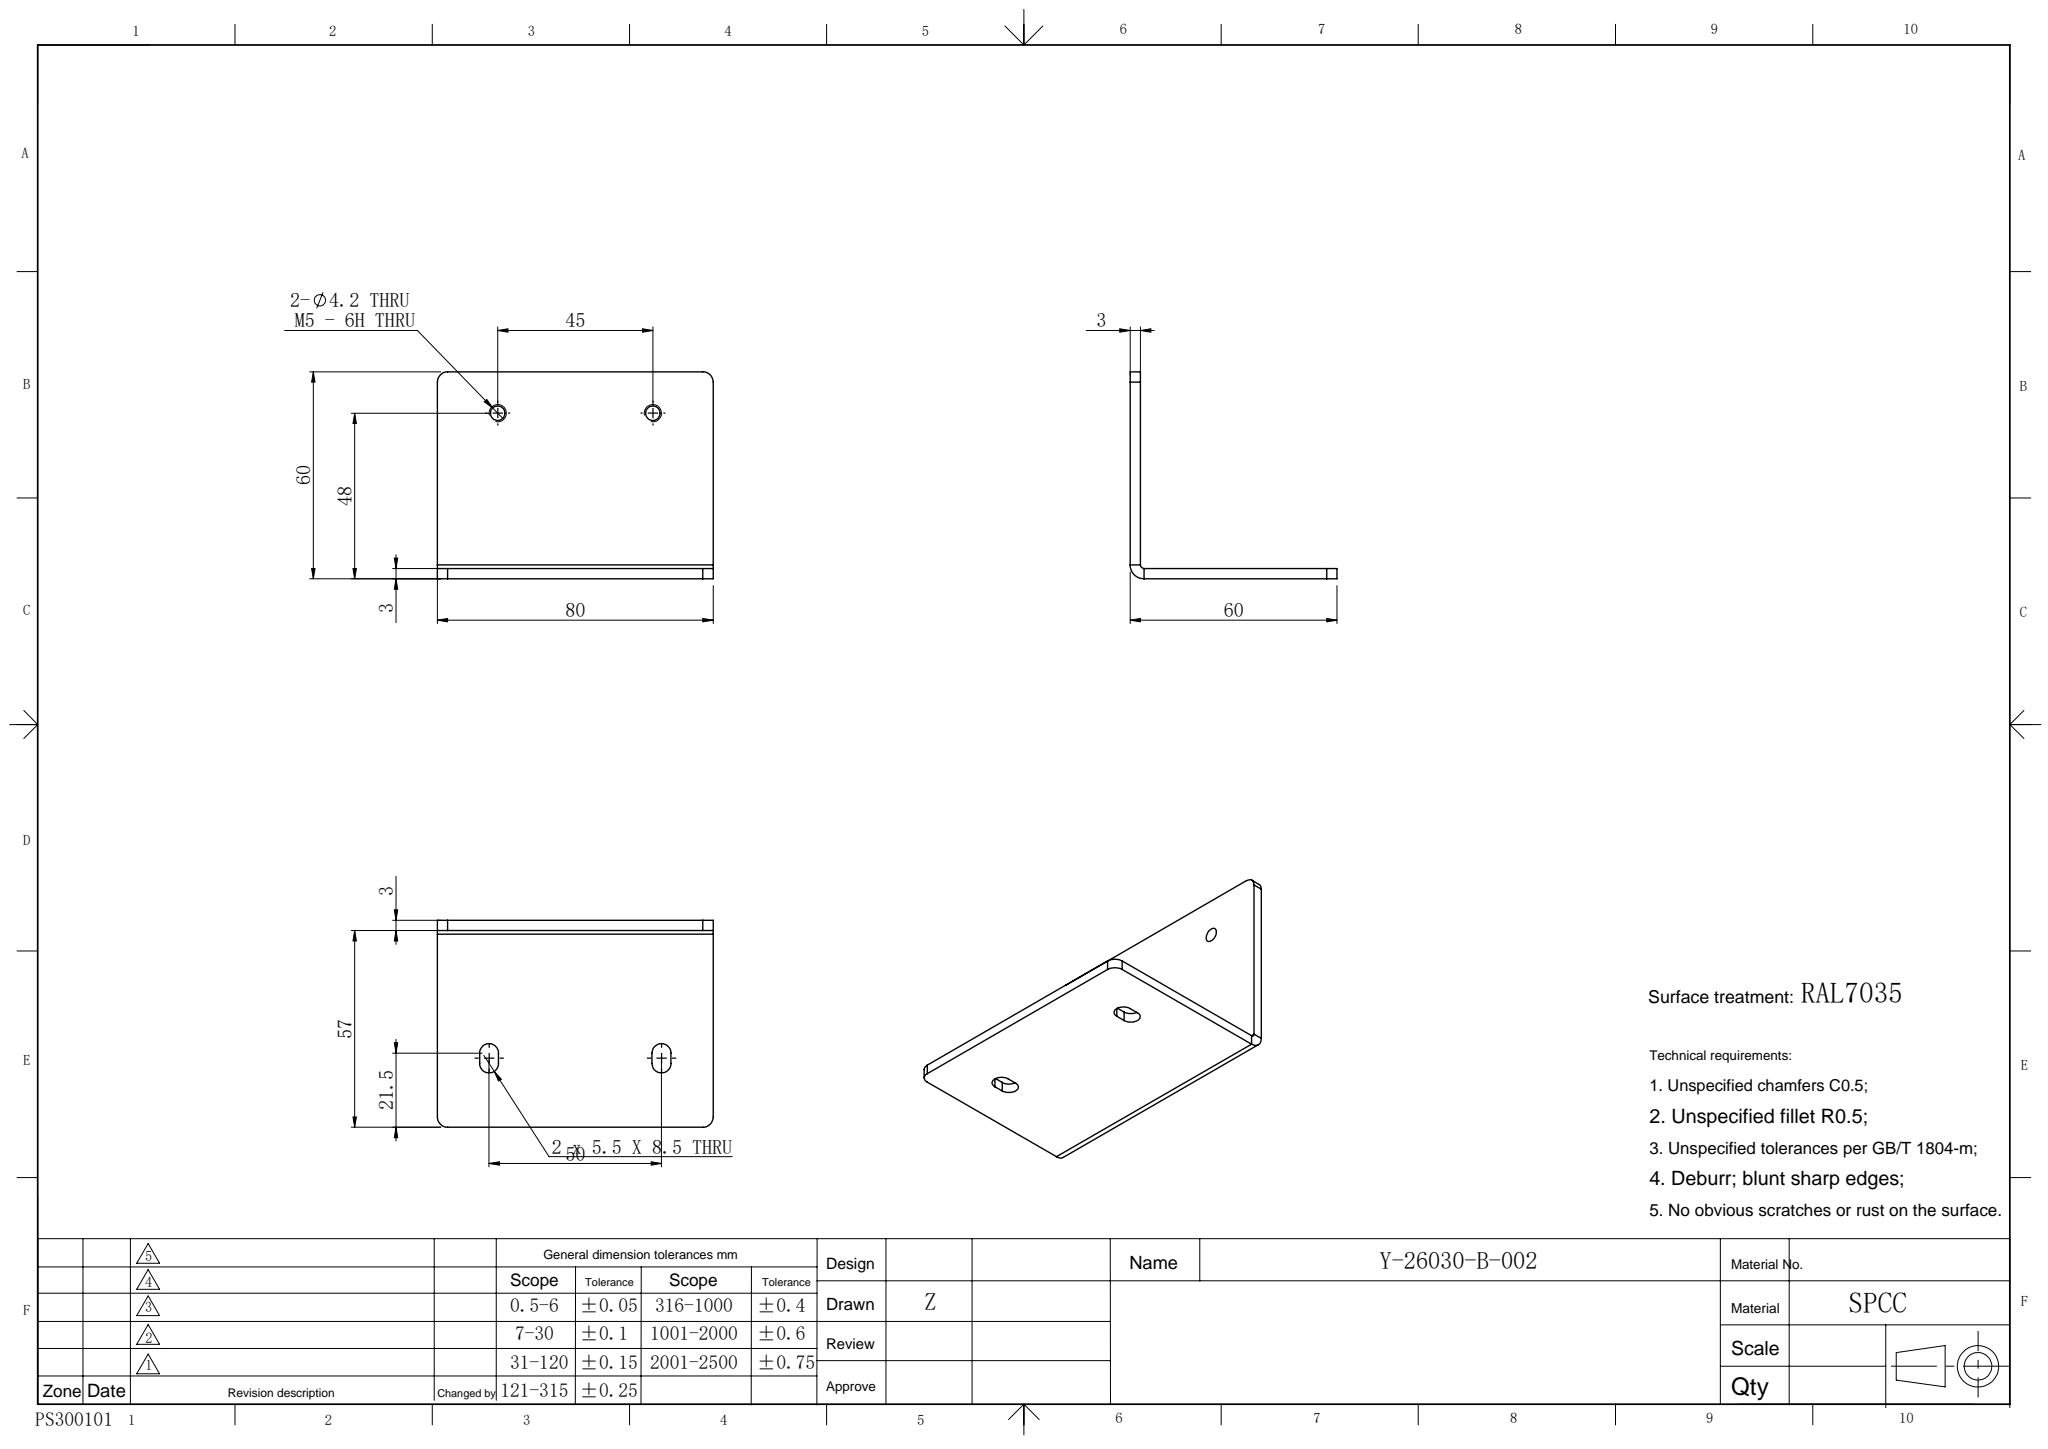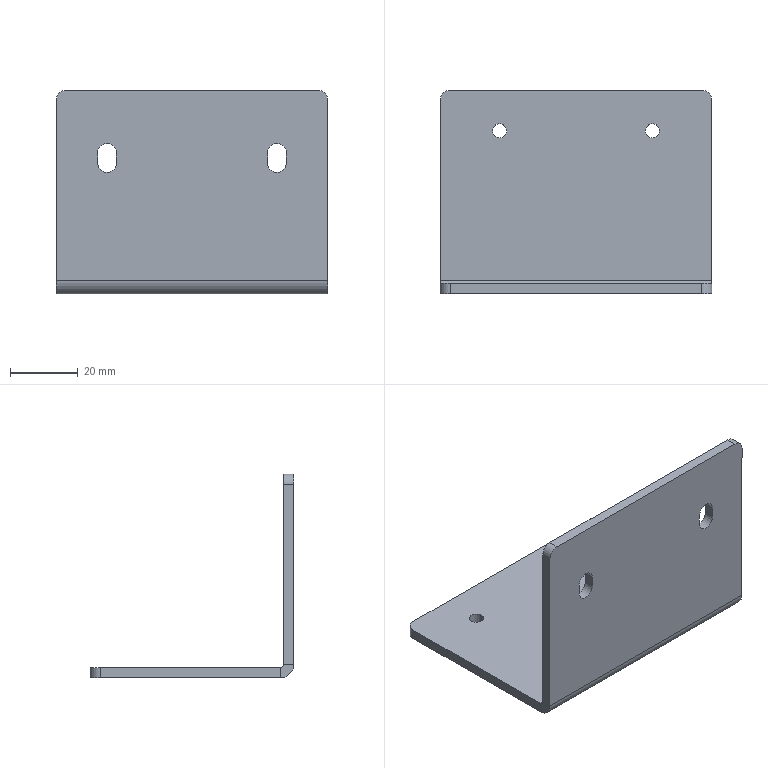Part | SolidWorks | features HoleWzd 2, EdgeFlange 1, Fillet 1, FlatPattern 1, SMBaseFlange 1, SheetMetal 1 | 1 solid | 32 faces | box 80 x 60 x 60 mm | volume 27475 mm3 | cylinder 16 | plane 16 | commonest cylinder face diameters 5.5 x6 4.2 x4 6 x4 2 x1 8 x1
STEP:
#1=CARTESIAN_POINT('',(-25.,-30.,41.25));
#2=VERTEX_POINT('',#1);
#3=CARTESIAN_POINT('',(-22.25,-30.,38.5));
#4=VERTEX_POINT('',#3);
#5=CARTESIAN_POINT('',(-25.,-30.,38.5));
#6=DIRECTION('',(0.,1.,0.));
#7=DIRECTION('',(0.,0.,1.));
#8=AXIS2_PLACEMENT_3D('',#5,#6,#7);
#9=CIRCLE('',#8,2.75);
#10=EDGE_CURVE('',#2,#4,#9,.T.);
#11=ORIENTED_EDGE('',*,*,#10,.F.);
#12=CARTESIAN_POINT('',(-25.,-27.,41.25));
#13=VERTEX_POINT('',#12);
#14=CARTESIAN_POINT('',(-25.,-27.,41.25));
#15=DIRECTION('',(0.,1.,0.));
#16=VECTOR('',#15,1000.);
#17=LINE('',#14,#16);
#18=EDGE_CURVE('',#2,#13,#17,.T.);
#19=ORIENTED_EDGE('',*,*,#18,.T.);
#20=CARTESIAN_POINT('',(-22.25,-27.,38.5));
#21=VERTEX_POINT('',#20);
#22=CARTESIAN_POINT('',(-25.,-27.,38.5));
#23=DIRECTION('',(0.,1.,0.));
#24=DIRECTION('',(0.,0.,1.));
#25=AXIS2_PLACEMENT_3D('',#22,#23,#24);
#26=CIRCLE('',#25,2.75);
#27=EDGE_CURVE('',#13,#21,#26,.T.);
#28=ORIENTED_EDGE('',*,*,#27,.T.);
#29=CARTESIAN_POINT('',(-22.25,-30.001,38.5));
#30=DIRECTION('',(0.,-1.,0.));
#31=VECTOR('',#30,1000.);
#32=LINE('',#29,#31);
#33=EDGE_CURVE('',#21,#4,#32,.T.);
#34=ORIENTED_EDGE('',*,*,#33,.T.);
#35=EDGE_LOOP('',(#11,#19,#28,#34));
#36=FACE_OUTER_BOUND('',#35,.T.);
#37=CARTESIAN_POINT('',(-25.,-27.,38.5));
#38=DIRECTION('',(0.,1.,0.));
#39=DIRECTION('',(0.,0.,1.));
#40=AXIS2_PLACEMENT_3D('',#37,#38,#39);
#41=CYLINDRICAL_SURFACE('',#40,2.75);
#42=ADVANCED_FACE('',(#36),#41,.F.);
#43=CARTESIAN_POINT('',(25.,-30.,41.25));
#44=VERTEX_POINT('',#43);
#45=CARTESIAN_POINT('',(27.75,-30.,38.5));
#46=VERTEX_POINT('',#45);
#47=CARTESIAN_POINT('',(25.,-30.,38.5));
#48=DIRECTION('',(0.,1.,0.));
#49=DIRECTION('',(0.,0.,1.));
#50=AXIS2_PLACEMENT_3D('',#47,#48,#49);
#51=CIRCLE('',#50,2.75);
#52=EDGE_CURVE('',#44,#46,#51,.T.);
#53=ORIENTED_EDGE('',*,*,#52,.F.);
#54=CARTESIAN_POINT('',(25.,-27.,41.25));
#55=VERTEX_POINT('',#54);
#56=CARTESIAN_POINT('',(25.,-27.,41.25));
#57=DIRECTION('',(0.,1.,0.));
#58=VECTOR('',#57,1000.);
#59=LINE('',#56,#58);
#60=EDGE_CURVE('',#44,#55,#59,.T.);
#61=ORIENTED_EDGE('',*,*,#60,.T.);
#62=CARTESIAN_POINT('',(27.75,-27.,38.5));
#63=VERTEX_POINT('',#62);
#64=CARTESIAN_POINT('',(25.,-27.,38.5));
#65=DIRECTION('',(0.,1.,0.));
#66=DIRECTION('',(0.,0.,1.));
#67=AXIS2_PLACEMENT_3D('',#64,#65,#66);
#68=CIRCLE('',#67,2.75);
#69=EDGE_CURVE('',#55,#63,#68,.T.);
#70=ORIENTED_EDGE('',*,*,#69,.T.);
#71=CARTESIAN_POINT('',(27.75,-30.001,38.5));
#72=DIRECTION('',(0.,-1.,0.));
#73=VECTOR('',#72,1000.);
#74=LINE('',#71,#73);
#75=EDGE_CURVE('',#63,#46,#74,.T.);
#76=ORIENTED_EDGE('',*,*,#75,.T.);
#77=EDGE_LOOP('',(#53,#61,#70,#76));
#78=FACE_OUTER_BOUND('',#77,.T.);
#79=CARTESIAN_POINT('',(25.,-27.,38.5));
#80=DIRECTION('',(0.,1.,0.));
#81=DIRECTION('',(0.,0.,1.));
#82=AXIS2_PLACEMENT_3D('',#79,#80,#81);
#83=CYLINDRICAL_SURFACE('',#82,2.75);
#84=ADVANCED_FACE('',(#78),#83,.F.);
#85=CARTESIAN_POINT('',(20.4,18.,0.));
#86=VERTEX_POINT('',#85);
#87=CARTESIAN_POINT('',(24.6,18.,0.));
#88=VERTEX_POINT('',#87);
#89=CARTESIAN_POINT('',(22.5,18.,0.));
#90=DIRECTION('',(0.,0.,1.));
#91=DIRECTION('',(1.,0.,0.));
#92=AXIS2_PLACEMENT_3D('',#89,#90,#91);
#93=CIRCLE('',#92,2.1);
#94=EDGE_CURVE('',#86,#88,#93,.T.);
#95=ORIENTED_EDGE('',*,*,#94,.T.);
#96=CARTESIAN_POINT('',(24.6,18.,-3.));
#97=VERTEX_POINT('',#96);
#98=CARTESIAN_POINT('',(24.6,18.,-3.));
#99=DIRECTION('',(0.,0.,-1.));
#100=VECTOR('',#99,1000.);
#101=LINE('',#98,#100);
#102=EDGE_CURVE('',#88,#97,#101,.T.);
#103=ORIENTED_EDGE('',*,*,#102,.T.);
#104=CARTESIAN_POINT('',(20.4,18.,-3.));
#105=VERTEX_POINT('',#104);
#106=CARTESIAN_POINT('',(22.5,18.,-3.));
#107=DIRECTION('',(0.,0.,-1.));
#108=DIRECTION('',(-1.,0.,0.));
#109=AXIS2_PLACEMENT_3D('',#106,#107,#108);
#110=CIRCLE('',#109,2.1);
#111=EDGE_CURVE('',#97,#105,#110,.T.);
#112=ORIENTED_EDGE('',*,*,#111,.T.);
#113=CARTESIAN_POINT('',(20.4,18.,-3.));
#114=DIRECTION('',(0.,0.,-1.));
#115=VECTOR('',#114,1000.);
#116=LINE('',#113,#115);
#117=EDGE_CURVE('',#86,#105,#116,.T.);
#118=ORIENTED_EDGE('',*,*,#117,.F.);
#119=EDGE_LOOP('',(#95,#103,#112,#118));
#120=FACE_OUTER_BOUND('',#119,.T.);
#121=CARTESIAN_POINT('',(22.5,18.,-3.));
#122=DIRECTION('',(0.,0.,-1.));
#123=DIRECTION('',(-1.,0.,0.));
#124=AXIS2_PLACEMENT_3D('',#121,#122,#123);
#125=CYLINDRICAL_SURFACE('',#124,2.1);
#126=ADVANCED_FACE('',(#120),#125,.F.);
#127=CARTESIAN_POINT('',(-24.6,18.,0.));
#128=VERTEX_POINT('',#127);
#129=CARTESIAN_POINT('',(-20.4,18.,0.));
#130=VERTEX_POINT('',#129);
#131=CARTESIAN_POINT('',(-22.5,18.,0.));
#132=DIRECTION('',(0.,0.,1.));
#133=DIRECTION('',(1.,0.,0.));
#134=AXIS2_PLACEMENT_3D('',#131,#132,#133);
#135=CIRCLE('',#134,2.1);
#136=EDGE_CURVE('',#128,#130,#135,.T.);
#137=ORIENTED_EDGE('',*,*,#136,.T.);
#138=CARTESIAN_POINT('',(-20.4,18.,-3.));
#139=VERTEX_POINT('',#138);
#140=CARTESIAN_POINT('',(-20.4,18.,-3.));
#141=DIRECTION('',(0.,0.,-1.));
#142=VECTOR('',#141,1000.);
#143=LINE('',#140,#142);
#144=EDGE_CURVE('',#130,#139,#143,.T.);
#145=ORIENTED_EDGE('',*,*,#144,.T.);
#146=CARTESIAN_POINT('',(-24.6,18.,-3.));
#147=VERTEX_POINT('',#146);
#148=CARTESIAN_POINT('',(-22.5,18.,-3.));
#149=DIRECTION('',(0.,0.,-1.));
#150=DIRECTION('',(-1.,0.,0.));
#151=AXIS2_PLACEMENT_3D('',#148,#149,#150);
#152=CIRCLE('',#151,2.1);
#153=EDGE_CURVE('',#139,#147,#152,.T.);
#154=ORIENTED_EDGE('',*,*,#153,.T.);
#155=CARTESIAN_POINT('',(-24.6,18.,-3.));
#156=DIRECTION('',(0.,0.,-1.));
#157=VECTOR('',#156,1000.);
#158=LINE('',#155,#157);
#159=EDGE_CURVE('',#128,#147,#158,.T.);
#160=ORIENTED_EDGE('',*,*,#159,.F.);
#161=EDGE_LOOP('',(#137,#145,#154,#160));
#162=FACE_OUTER_BOUND('',#161,.T.);
#163=CARTESIAN_POINT('',(-22.5,18.,-3.));
#164=DIRECTION('',(0.,0.,-1.));
#165=DIRECTION('',(-1.,0.,0.));
#166=AXIS2_PLACEMENT_3D('',#163,#164,#165);
#167=CYLINDRICAL_SURFACE('',#166,2.1);
#168=ADVANCED_FACE('',(#162),#167,.F.);
#169=CARTESIAN_POINT('',(40.,-26.,-3.));
#170=VERTEX_POINT('',#169);
#171=CARTESIAN_POINT('',(40.,27.,-3.));
#172=VERTEX_POINT('',#171);
#173=CARTESIAN_POINT('',(40.,-30.,-3.));
#174=DIRECTION('',(0.,1.,0.));
#175=VECTOR('',#174,1000.);
#176=LINE('',#173,#175);
#177=EDGE_CURVE('',#170,#172,#176,.T.);
#178=ORIENTED_EDGE('',*,*,#177,.T.);
#179=CARTESIAN_POINT('',(40.,27.,0.));
#180=VERTEX_POINT('',#179);
#181=CARTESIAN_POINT('',(40.,27.,-3.));
#182=DIRECTION('',(0.,0.,1.));
#183=VECTOR('',#182,1000.);
#184=LINE('',#181,#183);
#185=EDGE_CURVE('',#172,#180,#184,.T.);
#186=ORIENTED_EDGE('',*,*,#185,.T.);
#187=CARTESIAN_POINT('',(40.,-26.,0.));
#188=VERTEX_POINT('',#187);
#189=CARTESIAN_POINT('',(40.,-30.,0.));
#190=DIRECTION('',(0.,1.,0.));
#191=VECTOR('',#190,1000.);
#192=LINE('',#189,#191);
#193=EDGE_CURVE('',#188,#180,#192,.T.);
#194=ORIENTED_EDGE('',*,*,#193,.F.);
#195=CARTESIAN_POINT('',(40.,-26.,0.));
#196=DIRECTION('',(0.,0.,-1.));
#197=VECTOR('',#196,1000.);
#198=LINE('',#195,#197);
#199=EDGE_CURVE('',#188,#170,#198,.T.);
#200=ORIENTED_EDGE('',*,*,#199,.T.);
#201=EDGE_LOOP('',(#178,#186,#194,#200));
#202=FACE_OUTER_BOUND('',#201,.T.);
#203=CARTESIAN_POINT('',(40.,-30.,-3.));
#204=DIRECTION('',(1.,0.,0.));
#205=DIRECTION('',(0.,1.,0.));
#206=AXIS2_PLACEMENT_3D('',#203,#204,#205);
#207=PLANE('',#206);
#208=ADVANCED_FACE('',(#202),#207,.T.);
#209=CARTESIAN_POINT('',(22.5,18.,-3.));
#210=DIRECTION('',(0.,0.,-1.));
#211=DIRECTION('',(-1.,0.,0.));
#212=AXIS2_PLACEMENT_3D('',#209,#210,#211);
#213=CIRCLE('',#212,2.1);
#214=EDGE_CURVE('',#105,#97,#213,.T.);
#215=ORIENTED_EDGE('',*,*,#214,.F.);
#216=ORIENTED_EDGE('',*,*,#111,.F.);
#217=EDGE_LOOP('',(#215,#216));
#218=FACE_BOUND('',#217,.T.);
#219=CARTESIAN_POINT('',(-22.5,18.,-3.));
#220=DIRECTION('',(0.,0.,-1.));
#221=DIRECTION('',(-1.,0.,0.));
#222=AXIS2_PLACEMENT_3D('',#219,#220,#221);
#223=CIRCLE('',#222,2.1);
#224=EDGE_CURVE('',#147,#139,#223,.T.);
#225=ORIENTED_EDGE('',*,*,#224,.F.);
#226=ORIENTED_EDGE('',*,*,#153,.F.);
#227=EDGE_LOOP('',(#225,#226));
#228=FACE_BOUND('',#227,.T.);
#229=CARTESIAN_POINT('',(37.,30.,-3.));
#230=VERTEX_POINT('',#229);
#231=CARTESIAN_POINT('',(-37.,30.,-3.));
#232=VERTEX_POINT('',#231);
#233=CARTESIAN_POINT('',(40.,30.,-3.));
#234=DIRECTION('',(-1.,0.,0.));
#235=VECTOR('',#234,1000.);
#236=LINE('',#233,#235);
#237=EDGE_CURVE('',#230,#232,#236,.T.);
#238=ORIENTED_EDGE('',*,*,#237,.F.);
#239=CARTESIAN_POINT('',(37.,27.,-3.));
#240=DIRECTION('',(0.,0.,-1.));
#241=DIRECTION('',(1.,0.,0.));
#242=AXIS2_PLACEMENT_3D('',#239,#240,#241);
#243=CIRCLE('',#242,3.);
#244=EDGE_CURVE('',#230,#172,#243,.T.);
#245=ORIENTED_EDGE('',*,*,#244,.T.);
#246=ORIENTED_EDGE('',*,*,#177,.F.);
#247=CARTESIAN_POINT('',(-40.,-26.,-3.));
#248=VERTEX_POINT('',#247);
#249=CARTESIAN_POINT('',(40.,-26.,-3.));
#250=DIRECTION('',(-1.,0.,0.));
#251=VECTOR('',#250,1000.);
#252=LINE('',#249,#251);
#253=EDGE_CURVE('',#170,#248,#252,.T.);
#254=ORIENTED_EDGE('',*,*,#253,.T.);
#255=CARTESIAN_POINT('',(-40.,27.,-3.));
#256=VERTEX_POINT('',#255);
#257=CARTESIAN_POINT('',(-40.,-30.,-3.));
#258=DIRECTION('',(0.,-1.,0.));
#259=VECTOR('',#258,1000.);
#260=LINE('',#257,#259);
#261=EDGE_CURVE('',#256,#248,#260,.T.);
#262=ORIENTED_EDGE('',*,*,#261,.F.);
#263=CARTESIAN_POINT('',(-37.,27.,-3.));
#264=DIRECTION('',(0.,0.,-1.));
#265=DIRECTION('',(1.,0.,0.));
#266=AXIS2_PLACEMENT_3D('',#263,#264,#265);
#267=CIRCLE('',#266,3.);
#268=EDGE_CURVE('',#256,#232,#267,.T.);
#269=ORIENTED_EDGE('',*,*,#268,.T.);
#270=EDGE_LOOP('',(#238,#245,#246,#254,#262,#269));
#271=FACE_OUTER_BOUND('',#270,.T.);
#272=CARTESIAN_POINT('',(0.,0.,-3.));
#273=DIRECTION('',(0.,0.,1.));
#274=DIRECTION('',(1.,0.,0.));
#275=AXIS2_PLACEMENT_3D('',#272,#273,#274);
#276=PLANE('',#275);
#277=ADVANCED_FACE('',(#218,#228,#271),#276,.F.);
#278=ORIENTED_EDGE('',*,*,#94,.F.);
#279=CARTESIAN_POINT('',(22.5,18.,0.));
#280=DIRECTION('',(0.,0.,1.));
#281=DIRECTION('',(1.,0.,0.));
#282=AXIS2_PLACEMENT_3D('',#279,#280,#281);
#283=CIRCLE('',#282,2.1);
#284=EDGE_CURVE('',#88,#86,#283,.T.);
#285=ORIENTED_EDGE('',*,*,#284,.F.);
#286=EDGE_LOOP('',(#278,#285));
#287=FACE_BOUND('',#286,.T.);
#288=ORIENTED_EDGE('',*,*,#136,.F.);
#289=CARTESIAN_POINT('',(-22.5,18.,0.));
#290=DIRECTION('',(0.,0.,1.));
#291=DIRECTION('',(1.,0.,0.));
#292=AXIS2_PLACEMENT_3D('',#289,#290,#291);
#293=CIRCLE('',#292,2.1);
#294=EDGE_CURVE('',#130,#128,#293,.T.);
#295=ORIENTED_EDGE('',*,*,#294,.F.);
#296=EDGE_LOOP('',(#288,#295));
#297=FACE_BOUND('',#296,.T.);
#298=ORIENTED_EDGE('',*,*,#193,.T.);
#299=CARTESIAN_POINT('',(37.,30.,0.));
#300=VERTEX_POINT('',#299);
#301=CARTESIAN_POINT('',(37.,27.,0.));
#302=DIRECTION('',(0.,0.,1.));
#303=DIRECTION('',(1.,0.,0.));
#304=AXIS2_PLACEMENT_3D('',#301,#302,#303);
#305=CIRCLE('',#304,3.);
#306=EDGE_CURVE('',#180,#300,#305,.T.);
#307=ORIENTED_EDGE('',*,*,#306,.T.);
#308=CARTESIAN_POINT('',(-37.,30.,0.));
#309=VERTEX_POINT('',#308);
#310=CARTESIAN_POINT('',(40.,30.,0.));
#311=DIRECTION('',(-1.,0.,0.));
#312=VECTOR('',#311,1000.);
#313=LINE('',#310,#312);
#314=EDGE_CURVE('',#300,#309,#313,.T.);
#315=ORIENTED_EDGE('',*,*,#314,.T.);
#316=CARTESIAN_POINT('',(-40.,27.,0.));
#317=VERTEX_POINT('',#316);
#318=CARTESIAN_POINT('',(-37.,27.,0.));
#319=DIRECTION('',(0.,0.,1.));
#320=DIRECTION('',(1.,0.,0.));
#321=AXIS2_PLACEMENT_3D('',#318,#319,#320);
#322=CIRCLE('',#321,3.);
#323=EDGE_CURVE('',#309,#317,#322,.T.);
#324=ORIENTED_EDGE('',*,*,#323,.T.);
#325=CARTESIAN_POINT('',(-40.,-26.,0.));
#326=VERTEX_POINT('',#325);
#327=CARTESIAN_POINT('',(-40.,-30.,0.));
#328=DIRECTION('',(0.,-1.,0.));
#329=VECTOR('',#328,1000.);
#330=LINE('',#327,#329);
#331=EDGE_CURVE('',#317,#326,#330,.T.);
#332=ORIENTED_EDGE('',*,*,#331,.T.);
#333=CARTESIAN_POINT('',(40.,-26.,0.));
#334=DIRECTION('',(-1.,0.,0.));
#335=VECTOR('',#334,1000.);
#336=LINE('',#333,#335);
#337=EDGE_CURVE('',#188,#326,#336,.T.);
#338=ORIENTED_EDGE('',*,*,#337,.F.);
#339=EDGE_LOOP('',(#298,#307,#315,#324,#332,#338));
#340=FACE_OUTER_BOUND('',#339,.T.);
#341=CARTESIAN_POINT('',(0.,0.,0.));
#342=DIRECTION('',(0.,0.,1.));
#343=DIRECTION('',(1.,0.,0.));
#344=AXIS2_PLACEMENT_3D('',#341,#342,#343);
#345=PLANE('',#344);
#346=ADVANCED_FACE('',(#287,#297,#340),#345,.T.);
#347=ORIENTED_EDGE('',*,*,#331,.F.);
#348=CARTESIAN_POINT('',(-40.,27.,-3.));
#349=DIRECTION('',(0.,0.,-1.));
#350=VECTOR('',#349,1000.);
#351=LINE('',#348,#350);
#352=EDGE_CURVE('',#317,#256,#351,.T.);
#353=ORIENTED_EDGE('',*,*,#352,.T.);
#354=ORIENTED_EDGE('',*,*,#261,.T.);
#355=CARTESIAN_POINT('',(-40.,-26.,0.));
#356=DIRECTION('',(0.,0.,-1.));
#357=VECTOR('',#356,1000.);
#358=LINE('',#355,#357);
#359=EDGE_CURVE('',#326,#248,#358,.T.);
#360=ORIENTED_EDGE('',*,*,#359,.F.);
#361=EDGE_LOOP('',(#347,#353,#354,#360));
#362=FACE_OUTER_BOUND('',#361,.T.);
#363=CARTESIAN_POINT('',(-40.,-30.,-3.));
#364=DIRECTION('',(-1.,0.,0.));
#365=DIRECTION('',(0.,0.,1.));
#366=AXIS2_PLACEMENT_3D('',#363,#364,#365);
#367=PLANE('',#366);
#368=ADVANCED_FACE('',(#362),#367,.T.);
#369=ORIENTED_EDGE('',*,*,#314,.F.);
#370=CARTESIAN_POINT('',(37.,30.,-3.));
#371=DIRECTION('',(0.,0.,-1.));
#372=VECTOR('',#371,1000.);
#373=LINE('',#370,#372);
#374=EDGE_CURVE('',#300,#230,#373,.T.);
#375=ORIENTED_EDGE('',*,*,#374,.T.);
#376=ORIENTED_EDGE('',*,*,#237,.T.);
#377=CARTESIAN_POINT('',(-37.,30.,-3.));
#378=DIRECTION('',(0.,0.,1.));
#379=VECTOR('',#378,1000.);
#380=LINE('',#377,#379);
#381=EDGE_CURVE('',#232,#309,#380,.T.);
#382=ORIENTED_EDGE('',*,*,#381,.T.);
#383=EDGE_LOOP('',(#369,#375,#376,#382));
#384=FACE_OUTER_BOUND('',#383,.T.);
#385=CARTESIAN_POINT('',(40.,30.,-3.));
#386=DIRECTION('',(0.,1.,0.));
#387=DIRECTION('',(-1.,0.,0.));
#388=AXIS2_PLACEMENT_3D('',#385,#386,#387);
#389=PLANE('',#388);
#390=ADVANCED_FACE('',(#384),#389,.T.);
#391=CARTESIAN_POINT('',(-40.,-27.,1.));
#392=VERTEX_POINT('',#391);
#393=CARTESIAN_POINT('',(-40.,-30.,1.));
#394=VERTEX_POINT('',#393);
#395=CARTESIAN_POINT('',(-40.,-30.,1.));
#396=DIRECTION('',(0.,-1.,0.));
#397=VECTOR('',#396,1000.);
#398=LINE('',#395,#397);
#399=EDGE_CURVE('',#392,#394,#398,.T.);
#400=ORIENTED_EDGE('',*,*,#399,.F.);
#401=CARTESIAN_POINT('',(-40.,-26.,1.));
#402=DIRECTION('',(-1.,0.,0.));
#403=DIRECTION('',(0.,0.,-1.));
#404=AXIS2_PLACEMENT_3D('',#401,#402,#403);
#405=CIRCLE('',#404,1.);
#406=EDGE_CURVE('',#326,#392,#405,.T.);
#407=ORIENTED_EDGE('',*,*,#406,.F.);
#408=ORIENTED_EDGE('',*,*,#359,.T.);
#409=CARTESIAN_POINT('',(-40.,-26.,1.));
#410=DIRECTION('',(-1.,0.,0.));
#411=DIRECTION('',(0.,0.,-1.));
#412=AXIS2_PLACEMENT_3D('',#409,#410,#411);
#413=CIRCLE('',#412,4.);
#414=EDGE_CURVE('',#248,#394,#413,.T.);
#415=ORIENTED_EDGE('',*,*,#414,.T.);
#416=EDGE_LOOP('',(#400,#407,#408,#415));
#417=FACE_OUTER_BOUND('',#416,.T.);
#418=CARTESIAN_POINT('',(-40.,-26.,1.));
#419=DIRECTION('',(-1.,0.,0.));
#420=DIRECTION('',(0.,0.,1.));
#421=AXIS2_PLACEMENT_3D('',#418,#419,#420);
#422=PLANE('',#421);
#423=ADVANCED_FACE('',(#417),#422,.T.);
#424=CARTESIAN_POINT('',(40.,-27.,1.));
#425=VERTEX_POINT('',#424);
#426=CARTESIAN_POINT('',(40.,-26.,1.));
#427=DIRECTION('',(1.,0.,0.));
#428=DIRECTION('',(0.,0.,-1.));
#429=AXIS2_PLACEMENT_3D('',#426,#427,#428);
#430=CIRCLE('',#429,1.);
#431=EDGE_CURVE('',#425,#188,#430,.T.);
#432=ORIENTED_EDGE('',*,*,#431,.F.);
#433=CARTESIAN_POINT('',(40.,-30.,1.));
#434=VERTEX_POINT('',#433);
#435=CARTESIAN_POINT('',(40.,-27.,1.));
#436=DIRECTION('',(0.,-1.,0.));
#437=VECTOR('',#436,1000.);
#438=LINE('',#435,#437);
#439=EDGE_CURVE('',#425,#434,#438,.T.);
#440=ORIENTED_EDGE('',*,*,#439,.T.);
#441=CARTESIAN_POINT('',(40.,-26.,1.));
#442=DIRECTION('',(1.,0.,0.));
#443=DIRECTION('',(0.,0.,-1.));
#444=AXIS2_PLACEMENT_3D('',#441,#442,#443);
#445=CIRCLE('',#444,4.);
#446=EDGE_CURVE('',#434,#170,#445,.T.);
#447=ORIENTED_EDGE('',*,*,#446,.T.);
#448=ORIENTED_EDGE('',*,*,#199,.F.);
#449=EDGE_LOOP('',(#432,#440,#447,#448));
#450=FACE_OUTER_BOUND('',#449,.T.);
#451=CARTESIAN_POINT('',(40.,-26.,1.));
#452=DIRECTION('',(-1.,0.,0.));
#453=DIRECTION('',(0.,0.,1.));
#454=AXIS2_PLACEMENT_3D('',#451,#452,#453);
#455=PLANE('',#454);
#456=ADVANCED_FACE('',(#450),#455,.F.);
#457=ORIENTED_EDGE('',*,*,#253,.F.);
#458=ORIENTED_EDGE('',*,*,#446,.F.);
#459=CARTESIAN_POINT('',(-40.,-30.,1.));
#460=DIRECTION('',(-1.,0.,0.));
#461=VECTOR('',#460,1000.);
#462=LINE('',#459,#461);
#463=EDGE_CURVE('',#434,#394,#462,.T.);
#464=ORIENTED_EDGE('',*,*,#463,.T.);
#465=ORIENTED_EDGE('',*,*,#414,.F.);
#466=EDGE_LOOP('',(#457,#458,#464,#465));
#467=FACE_OUTER_BOUND('',#466,.T.);
#468=CARTESIAN_POINT('',(40.,-26.,1.));
#469=DIRECTION('',(1.,0.,0.));
#470=DIRECTION('',(0.,-1.,0.));
#471=AXIS2_PLACEMENT_3D('',#468,#469,#470);
#472=CYLINDRICAL_SURFACE('',#471,4.);
#473=ADVANCED_FACE('',(#467),#472,.T.);
#474=ORIENTED_EDGE('',*,*,#337,.T.);
#475=ORIENTED_EDGE('',*,*,#406,.T.);
#476=CARTESIAN_POINT('',(-40.,-27.,1.));
#477=DIRECTION('',(1.,0.,0.));
#478=VECTOR('',#477,1000.);
#479=LINE('',#476,#478);
#480=EDGE_CURVE('',#392,#425,#479,.T.);
#481=ORIENTED_EDGE('',*,*,#480,.T.);
#482=ORIENTED_EDGE('',*,*,#431,.T.);
#483=EDGE_LOOP('',(#474,#475,#481,#482));
#484=FACE_OUTER_BOUND('',#483,.T.);
#485=CARTESIAN_POINT('',(40.,-26.,1.));
#486=DIRECTION('',(1.,0.,0.));
#487=DIRECTION('',(0.,-1.,0.));
#488=AXIS2_PLACEMENT_3D('',#485,#486,#487);
#489=CYLINDRICAL_SURFACE('',#488,1.);
#490=ADVANCED_FACE('',(#484),#489,.F.);
#491=CARTESIAN_POINT('',(40.,-27.,54.));
#492=VERTEX_POINT('',#491);
#493=CARTESIAN_POINT('',(40.,-27.,57.));
#494=DIRECTION('',(0.,0.,1.));
#495=VECTOR('',#494,1000.);
#496=LINE('',#493,#495);
#497=EDGE_CURVE('',#425,#492,#496,.T.);
#498=ORIENTED_EDGE('',*,*,#497,.T.);
#499=CARTESIAN_POINT('',(40.,-30.,54.));
#500=VERTEX_POINT('',#499);
#501=CARTESIAN_POINT('',(40.,-30.,54.));
#502=DIRECTION('',(0.,-1.,0.));
#503=VECTOR('',#502,1000.);
#504=LINE('',#501,#503);
#505=EDGE_CURVE('',#492,#500,#504,.T.);
#506=ORIENTED_EDGE('',*,*,#505,.T.);
#507=CARTESIAN_POINT('',(40.,-30.,0.));
#508=DIRECTION('',(0.,0.,1.));
#509=VECTOR('',#508,1000.);
#510=LINE('',#507,#509);
#511=EDGE_CURVE('',#434,#500,#510,.T.);
#512=ORIENTED_EDGE('',*,*,#511,.F.);
#513=ORIENTED_EDGE('',*,*,#439,.F.);
#514=EDGE_LOOP('',(#498,#506,#512,#513));
#515=FACE_OUTER_BOUND('',#514,.T.);
#516=CARTESIAN_POINT('',(40.,-30.,57.));
#517=DIRECTION('',(-1.,0.,0.));
#518=DIRECTION('',(0.,-1.,0.));
#519=AXIS2_PLACEMENT_3D('',#516,#517,#518);
#520=PLANE('',#519);
#521=ADVANCED_FACE('',(#515),#520,.F.);
#522=CARTESIAN_POINT('',(-40.,-30.,54.));
#523=VERTEX_POINT('',#522);
#524=CARTESIAN_POINT('',(-40.,-30.,0.));
#525=DIRECTION('',(0.,0.,-1.));
#526=VECTOR('',#525,1000.);
#527=LINE('',#524,#526);
#528=EDGE_CURVE('',#523,#394,#527,.T.);
#529=ORIENTED_EDGE('',*,*,#528,.F.);
#530=CARTESIAN_POINT('',(-40.,-27.,54.));
#531=VERTEX_POINT('',#530);
#532=CARTESIAN_POINT('',(-40.,-30.,54.));
#533=DIRECTION('',(0.,1.,0.));
#534=VECTOR('',#533,1000.);
#535=LINE('',#532,#534);
#536=EDGE_CURVE('',#523,#531,#535,.T.);
#537=ORIENTED_EDGE('',*,*,#536,.T.);
#538=CARTESIAN_POINT('',(-40.,-27.,0.));
#539=DIRECTION('',(0.,0.,-1.));
#540=VECTOR('',#539,1000.);
#541=LINE('',#538,#540);
#542=EDGE_CURVE('',#531,#392,#541,.T.);
#543=ORIENTED_EDGE('',*,*,#542,.T.);
#544=ORIENTED_EDGE('',*,*,#399,.T.);
#545=EDGE_LOOP('',(#529,#537,#543,#544));
#546=FACE_OUTER_BOUND('',#545,.T.);
#547=CARTESIAN_POINT('',(-40.,-30.,0.));
#548=DIRECTION('',(1.,0.,0.));
#549=DIRECTION('',(0.,1.,0.));
#550=AXIS2_PLACEMENT_3D('',#547,#548,#549);
#551=PLANE('',#550);
#552=ADVANCED_FACE('',(#546),#551,.F.);
#553=CARTESIAN_POINT('',(-22.25,-30.,35.5));
#554=VERTEX_POINT('',#553);
#555=CARTESIAN_POINT('',(-27.75,-30.,35.5));
#556=VERTEX_POINT('',#555);
#557=CARTESIAN_POINT('',(-25.,-30.,35.5));
#558=DIRECTION('',(0.,1.,0.));
#559=DIRECTION('',(0.,0.,1.));
#560=AXIS2_PLACEMENT_3D('',#557,#558,#559);
#561=CIRCLE('',#560,2.75);
#562=EDGE_CURVE('',#554,#556,#561,.T.);
#563=ORIENTED_EDGE('',*,*,#562,.T.);
#564=CARTESIAN_POINT('',(-27.75,-30.,38.5));
#565=VERTEX_POINT('',#564);
#566=CARTESIAN_POINT('',(-27.75,-30.,0.));
#567=DIRECTION('',(0.,0.,1.));
#568=VECTOR('',#567,1000.);
#569=LINE('',#566,#568);
#570=EDGE_CURVE('',#556,#565,#569,.T.);
#571=ORIENTED_EDGE('',*,*,#570,.T.);
#572=CARTESIAN_POINT('',(-25.,-30.,38.5));
#573=DIRECTION('',(0.,1.,0.));
#574=DIRECTION('',(0.,0.,1.));
#575=AXIS2_PLACEMENT_3D('',#572,#573,#574);
#576=CIRCLE('',#575,2.75);
#577=EDGE_CURVE('',#565,#2,#576,.T.);
#578=ORIENTED_EDGE('',*,*,#577,.T.);
#579=ORIENTED_EDGE('',*,*,#10,.T.);
#580=CARTESIAN_POINT('',(-22.25,-30.,0.));
#581=DIRECTION('',(0.,0.,-1.));
#582=VECTOR('',#581,1000.);
#583=LINE('',#580,#582);
#584=EDGE_CURVE('',#4,#554,#583,.T.);
#585=ORIENTED_EDGE('',*,*,#584,.T.);
#586=EDGE_LOOP('',(#563,#571,#578,#579,#585));
#587=FACE_BOUND('',#586,.T.);
#588=CARTESIAN_POINT('',(27.75,-30.,35.5));
#589=VERTEX_POINT('',#588);
#590=CARTESIAN_POINT('',(22.25,-30.,35.5));
#591=VERTEX_POINT('',#590);
#592=CARTESIAN_POINT('',(25.,-30.,35.5));
#593=DIRECTION('',(0.,1.,0.));
#594=DIRECTION('',(0.,0.,1.));
#595=AXIS2_PLACEMENT_3D('',#592,#593,#594);
#596=CIRCLE('',#595,2.75);
#597=EDGE_CURVE('',#589,#591,#596,.T.);
#598=ORIENTED_EDGE('',*,*,#597,.T.);
#599=CARTESIAN_POINT('',(22.25,-30.,38.5));
#600=VERTEX_POINT('',#599);
#601=CARTESIAN_POINT('',(22.25,-30.,0.));
#602=DIRECTION('',(0.,0.,1.));
#603=VECTOR('',#602,1000.);
#604=LINE('',#601,#603);
#605=EDGE_CURVE('',#591,#600,#604,.T.);
#606=ORIENTED_EDGE('',*,*,#605,.T.);
#607=CARTESIAN_POINT('',(25.,-30.,38.5));
#608=DIRECTION('',(0.,1.,0.));
#609=DIRECTION('',(0.,0.,1.));
#610=AXIS2_PLACEMENT_3D('',#607,#608,#609);
#611=CIRCLE('',#610,2.75);
#612=EDGE_CURVE('',#600,#44,#611,.T.);
#613=ORIENTED_EDGE('',*,*,#612,.T.);
#614=ORIENTED_EDGE('',*,*,#52,.T.);
#615=CARTESIAN_POINT('',(27.75,-30.,0.));
#616=DIRECTION('',(0.,0.,-1.));
#617=VECTOR('',#616,1000.);
#618=LINE('',#615,#617);
#619=EDGE_CURVE('',#46,#589,#618,.T.);
#620=ORIENTED_EDGE('',*,*,#619,.T.);
#621=EDGE_LOOP('',(#598,#606,#613,#614,#620));
#622=FACE_BOUND('',#621,.T.);
#623=CARTESIAN_POINT('',(37.,-30.,57.));
#624=VERTEX_POINT('',#623);
#625=CARTESIAN_POINT('',(-37.,-30.,57.));
#626=VERTEX_POINT('',#625);
#627=CARTESIAN_POINT('',(0.,-30.,57.));
#628=DIRECTION('',(-1.,0.,0.));
#629=VECTOR('',#628,1000.);
#630=LINE('',#627,#629);
#631=EDGE_CURVE('',#624,#626,#630,.T.);
#632=ORIENTED_EDGE('',*,*,#631,.T.);
#633=CARTESIAN_POINT('',(-37.,-30.,54.));
#634=DIRECTION('',(0.,-1.,0.));
#635=DIRECTION('',(0.,0.,1.));
#636=AXIS2_PLACEMENT_3D('',#633,#634,#635);
#637=CIRCLE('',#636,3.);
#638=EDGE_CURVE('',#626,#523,#637,.T.);
#639=ORIENTED_EDGE('',*,*,#638,.T.);
#640=ORIENTED_EDGE('',*,*,#528,.T.);
#641=ORIENTED_EDGE('',*,*,#463,.F.);
#642=ORIENTED_EDGE('',*,*,#511,.T.);
#643=CARTESIAN_POINT('',(37.,-30.,54.));
#644=DIRECTION('',(0.,-1.,0.));
#645=DIRECTION('',(0.,0.,1.));
#646=AXIS2_PLACEMENT_3D('',#643,#644,#645);
#647=CIRCLE('',#646,3.);
#648=EDGE_CURVE('',#500,#624,#647,.T.);
#649=ORIENTED_EDGE('',*,*,#648,.T.);
#650=EDGE_LOOP('',(#632,#639,#640,#641,#642,#649));
#651=FACE_OUTER_BOUND('',#650,.T.);
#652=CARTESIAN_POINT('',(0.,-30.,0.));
#653=DIRECTION('',(0.,1.,0.));
#654=DIRECTION('',(0.,0.,1.));
#655=AXIS2_PLACEMENT_3D('',#652,#653,#654);
#656=PLANE('',#655);
#657=ADVANCED_FACE('',(#587,#622,#651),#656,.F.);
#658=CARTESIAN_POINT('',(-22.25,-27.,35.5));
#659=VERTEX_POINT('',#658);
#660=CARTESIAN_POINT('',(-27.75,-27.,35.5));
#661=VERTEX_POINT('',#660);
#662=CARTESIAN_POINT('',(-25.,-27.,35.5));
#663=DIRECTION('',(0.,1.,0.));
#664=DIRECTION('',(0.,0.,1.));
#665=AXIS2_PLACEMENT_3D('',#662,#663,#664);
#666=CIRCLE('',#665,2.75);
#667=EDGE_CURVE('',#659,#661,#666,.T.);
#668=ORIENTED_EDGE('',*,*,#667,.F.);
#669=CARTESIAN_POINT('',(-22.25,-27.,38.5));
#670=DIRECTION('',(0.,0.,-1.));
#671=VECTOR('',#670,1000.);
#672=LINE('',#669,#671);
#673=EDGE_CURVE('',#21,#659,#672,.T.);
#674=ORIENTED_EDGE('',*,*,#673,.F.);
#675=ORIENTED_EDGE('',*,*,#27,.F.);
#676=CARTESIAN_POINT('',(-27.75,-27.,38.5));
#677=VERTEX_POINT('',#676);
#678=CARTESIAN_POINT('',(-25.,-27.,38.5));
#679=DIRECTION('',(0.,1.,0.));
#680=DIRECTION('',(0.,0.,1.));
#681=AXIS2_PLACEMENT_3D('',#678,#679,#680);
#682=CIRCLE('',#681,2.75);
#683=EDGE_CURVE('',#677,#13,#682,.T.);
#684=ORIENTED_EDGE('',*,*,#683,.F.);
#685=CARTESIAN_POINT('',(-27.75,-27.,38.5));
#686=DIRECTION('',(0.,0.,-1.));
#687=VECTOR('',#686,1000.);
#688=LINE('',#685,#687);
#689=EDGE_CURVE('',#677,#661,#688,.T.);
#690=ORIENTED_EDGE('',*,*,#689,.T.);
#691=EDGE_LOOP('',(#668,#674,#675,#684,#690));
#692=FACE_BOUND('',#691,.T.);
#693=CARTESIAN_POINT('',(27.75,-27.,35.5));
#694=VERTEX_POINT('',#693);
#695=CARTESIAN_POINT('',(27.75,-27.,38.5));
#696=DIRECTION('',(0.,0.,-1.));
#697=VECTOR('',#696,1000.);
#698=LINE('',#695,#697);
#699=EDGE_CURVE('',#63,#694,#698,.T.);
#700=ORIENTED_EDGE('',*,*,#699,.F.);
#701=ORIENTED_EDGE('',*,*,#69,.F.);
#702=CARTESIAN_POINT('',(22.25,-27.,38.5));
#703=VERTEX_POINT('',#702);
#704=CARTESIAN_POINT('',(25.,-27.,38.5));
#705=DIRECTION('',(0.,1.,0.));
#706=DIRECTION('',(0.,0.,1.));
#707=AXIS2_PLACEMENT_3D('',#704,#705,#706);
#708=CIRCLE('',#707,2.75);
#709=EDGE_CURVE('',#703,#55,#708,.T.);
#710=ORIENTED_EDGE('',*,*,#709,.F.);
#711=CARTESIAN_POINT('',(22.25,-27.,35.5));
#712=VERTEX_POINT('',#711);
#713=CARTESIAN_POINT('',(22.25,-27.,38.5));
#714=DIRECTION('',(0.,0.,-1.));
#715=VECTOR('',#714,1000.);
#716=LINE('',#713,#715);
#717=EDGE_CURVE('',#703,#712,#716,.T.);
#718=ORIENTED_EDGE('',*,*,#717,.T.);
#719=CARTESIAN_POINT('',(25.,-27.,35.5));
#720=DIRECTION('',(0.,1.,0.));
#721=DIRECTION('',(0.,0.,1.));
#722=AXIS2_PLACEMENT_3D('',#719,#720,#721);
#723=CIRCLE('',#722,2.75);
#724=EDGE_CURVE('',#694,#712,#723,.T.);
#725=ORIENTED_EDGE('',*,*,#724,.F.);
#726=EDGE_LOOP('',(#700,#701,#710,#718,#725));
#727=FACE_BOUND('',#726,.T.);
#728=ORIENTED_EDGE('',*,*,#542,.F.);
#729=CARTESIAN_POINT('',(-37.,-27.,57.));
#730=VERTEX_POINT('',#729);
#731=CARTESIAN_POINT('',(-37.,-27.,54.));
#732=DIRECTION('',(0.,1.,0.));
#733=DIRECTION('',(0.,0.,1.));
#734=AXIS2_PLACEMENT_3D('',#731,#732,#733);
#735=CIRCLE('',#734,3.);
#736=EDGE_CURVE('',#531,#730,#735,.T.);
#737=ORIENTED_EDGE('',*,*,#736,.T.);
#738=CARTESIAN_POINT('',(37.,-27.,57.));
#739=VERTEX_POINT('',#738);
#740=CARTESIAN_POINT('',(-40.,-27.,57.));
#741=DIRECTION('',(-1.,0.,0.));
#742=VECTOR('',#741,1000.);
#743=LINE('',#740,#742);
#744=EDGE_CURVE('',#739,#730,#743,.T.);
#745=ORIENTED_EDGE('',*,*,#744,.F.);
#746=CARTESIAN_POINT('',(37.,-27.,54.));
#747=DIRECTION('',(0.,1.,0.));
#748=DIRECTION('',(0.,0.,1.));
#749=AXIS2_PLACEMENT_3D('',#746,#747,#748);
#750=CIRCLE('',#749,3.);
#751=EDGE_CURVE('',#739,#492,#750,.T.);
#752=ORIENTED_EDGE('',*,*,#751,.T.);
#753=ORIENTED_EDGE('',*,*,#497,.F.);
#754=ORIENTED_EDGE('',*,*,#480,.F.);
#755=EDGE_LOOP('',(#728,#737,#745,#752,#753,#754));
#756=FACE_OUTER_BOUND('',#755,.T.);
#757=CARTESIAN_POINT('',(0.,-27.,0.));
#758=DIRECTION('',(0.,1.,0.));
#759=DIRECTION('',(0.,0.,1.));
#760=AXIS2_PLACEMENT_3D('',#757,#758,#759);
#761=PLANE('',#760);
#762=ADVANCED_FACE('',(#692,#727,#756),#761,.T.);
#763=ORIENTED_EDGE('',*,*,#744,.T.);
#764=CARTESIAN_POINT('',(-37.,-30.,57.));
#765=DIRECTION('',(0.,-1.,0.));
#766=VECTOR('',#765,1000.);
#767=LINE('',#764,#766);
#768=EDGE_CURVE('',#730,#626,#767,.T.);
#769=ORIENTED_EDGE('',*,*,#768,.T.);
#770=ORIENTED_EDGE('',*,*,#631,.F.);
#771=CARTESIAN_POINT('',(37.,-30.,57.));
#772=DIRECTION('',(0.,1.,0.));
#773=VECTOR('',#772,1000.);
#774=LINE('',#771,#773);
#775=EDGE_CURVE('',#624,#739,#774,.T.);
#776=ORIENTED_EDGE('',*,*,#775,.T.);
#777=EDGE_LOOP('',(#763,#769,#770,#776));
#778=FACE_OUTER_BOUND('',#777,.T.);
#779=CARTESIAN_POINT('',(-40.,-30.,57.));
#780=DIRECTION('',(0.,0.,-1.));
#781=DIRECTION('',(0.,1.,0.));
#782=AXIS2_PLACEMENT_3D('',#779,#780,#781);
#783=PLANE('',#782);
#784=ADVANCED_FACE('',(#778),#783,.F.);
#785=ORIENTED_EDGE('',*,*,#638,.F.);
#786=ORIENTED_EDGE('',*,*,#768,.F.);
#787=ORIENTED_EDGE('',*,*,#736,.F.);
#788=ORIENTED_EDGE('',*,*,#536,.F.);
#789=EDGE_LOOP('',(#785,#786,#787,#788));
#790=FACE_OUTER_BOUND('',#789,.T.);
#791=CARTESIAN_POINT('',(-37.,-30.,54.));
#792=DIRECTION('',(0.,1.,0.));
#793=DIRECTION('',(0.,0.,1.));
#794=AXIS2_PLACEMENT_3D('',#791,#792,#793);
#795=CYLINDRICAL_SURFACE('',#794,3.);
#796=ADVANCED_FACE('',(#790),#795,.T.);
#797=ORIENTED_EDGE('',*,*,#648,.F.);
#798=ORIENTED_EDGE('',*,*,#505,.F.);
#799=ORIENTED_EDGE('',*,*,#751,.F.);
#800=ORIENTED_EDGE('',*,*,#775,.F.);
#801=EDGE_LOOP('',(#797,#798,#799,#800));
#802=FACE_OUTER_BOUND('',#801,.T.);
#803=CARTESIAN_POINT('',(37.,-30.,54.));
#804=DIRECTION('',(0.,1.,0.));
#805=DIRECTION('',(0.,0.,1.));
#806=AXIS2_PLACEMENT_3D('',#803,#804,#805);
#807=CYLINDRICAL_SURFACE('',#806,3.);
#808=ADVANCED_FACE('',(#802),#807,.T.);
#809=ORIENTED_EDGE('',*,*,#244,.F.);
#810=ORIENTED_EDGE('',*,*,#374,.F.);
#811=ORIENTED_EDGE('',*,*,#306,.F.);
#812=ORIENTED_EDGE('',*,*,#185,.F.);
#813=EDGE_LOOP('',(#809,#810,#811,#812));
#814=FACE_OUTER_BOUND('',#813,.T.);
#815=CARTESIAN_POINT('',(37.,27.,-3.));
#816=DIRECTION('',(0.,0.,1.));
#817=DIRECTION('',(1.,0.,0.));
#818=AXIS2_PLACEMENT_3D('',#815,#816,#817);
#819=CYLINDRICAL_SURFACE('',#818,3.);
#820=ADVANCED_FACE('',(#814),#819,.T.);
#821=ORIENTED_EDGE('',*,*,#268,.F.);
#822=ORIENTED_EDGE('',*,*,#352,.F.);
#823=ORIENTED_EDGE('',*,*,#323,.F.);
#824=ORIENTED_EDGE('',*,*,#381,.F.);
#825=EDGE_LOOP('',(#821,#822,#823,#824));
#826=FACE_OUTER_BOUND('',#825,.T.);
#827=CARTESIAN_POINT('',(-37.,27.,-3.));
#828=DIRECTION('',(0.,0.,1.));
#829=DIRECTION('',(1.,0.,0.));
#830=AXIS2_PLACEMENT_3D('',#827,#828,#829);
#831=CYLINDRICAL_SURFACE('',#830,3.);
#832=ADVANCED_FACE('',(#826),#831,.T.);
#833=ORIENTED_EDGE('',*,*,#144,.F.);
#834=ORIENTED_EDGE('',*,*,#294,.T.);
#835=ORIENTED_EDGE('',*,*,#159,.T.);
#836=ORIENTED_EDGE('',*,*,#224,.T.);
#837=EDGE_LOOP('',(#833,#834,#835,#836));
#838=FACE_OUTER_BOUND('',#837,.T.);
#839=CARTESIAN_POINT('',(-22.5,18.,-3.));
#840=DIRECTION('',(0.,0.,-1.));
#841=DIRECTION('',(-1.,0.,0.));
#842=AXIS2_PLACEMENT_3D('',#839,#840,#841);
#843=CYLINDRICAL_SURFACE('',#842,2.1);
#844=ADVANCED_FACE('',(#838),#843,.F.);
#845=ORIENTED_EDGE('',*,*,#102,.F.);
#846=ORIENTED_EDGE('',*,*,#284,.T.);
#847=ORIENTED_EDGE('',*,*,#117,.T.);
#848=ORIENTED_EDGE('',*,*,#214,.T.);
#849=EDGE_LOOP('',(#845,#846,#847,#848));
#850=FACE_OUTER_BOUND('',#849,.T.);
#851=CARTESIAN_POINT('',(22.5,18.,-3.));
#852=DIRECTION('',(0.,0.,-1.));
#853=DIRECTION('',(-1.,0.,0.));
#854=AXIS2_PLACEMENT_3D('',#851,#852,#853);
#855=CYLINDRICAL_SURFACE('',#854,2.1);
#856=ADVANCED_FACE('',(#850),#855,.F.);
#857=CARTESIAN_POINT('',(27.75,-30.001,35.5));
#858=DIRECTION('',(0.,-1.,0.));
#859=VECTOR('',#858,1000.);
#860=LINE('',#857,#859);
#861=EDGE_CURVE('',#694,#589,#860,.T.);
#862=ORIENTED_EDGE('',*,*,#861,.F.);
#863=ORIENTED_EDGE('',*,*,#724,.T.);
#864=CARTESIAN_POINT('',(22.25,-27.,35.5));
#865=DIRECTION('',(0.,1.,0.));
#866=VECTOR('',#865,1000.);
#867=LINE('',#864,#866);
#868=EDGE_CURVE('',#591,#712,#867,.T.);
#869=ORIENTED_EDGE('',*,*,#868,.F.);
#870=ORIENTED_EDGE('',*,*,#597,.F.);
#871=EDGE_LOOP('',(#862,#863,#869,#870));
#872=FACE_OUTER_BOUND('',#871,.T.);
#873=CARTESIAN_POINT('',(25.,-27.,35.5));
#874=DIRECTION('',(0.,1.,0.));
#875=DIRECTION('',(0.,0.,1.));
#876=AXIS2_PLACEMENT_3D('',#873,#874,#875);
#877=CYLINDRICAL_SURFACE('',#876,2.75);
#878=ADVANCED_FACE('',(#872),#877,.F.);
#879=ORIENTED_EDGE('',*,*,#60,.F.);
#880=ORIENTED_EDGE('',*,*,#612,.F.);
#881=CARTESIAN_POINT('',(22.25,-27.,38.5));
#882=DIRECTION('',(0.,-1.,0.));
#883=VECTOR('',#882,1000.);
#884=LINE('',#881,#883);
#885=EDGE_CURVE('',#703,#600,#884,.T.);
#886=ORIENTED_EDGE('',*,*,#885,.F.);
#887=ORIENTED_EDGE('',*,*,#709,.T.);
#888=EDGE_LOOP('',(#879,#880,#886,#887));
#889=FACE_OUTER_BOUND('',#888,.T.);
#890=CARTESIAN_POINT('',(25.,-27.,38.5));
#891=DIRECTION('',(0.,1.,0.));
#892=DIRECTION('',(0.,0.,1.));
#893=AXIS2_PLACEMENT_3D('',#890,#891,#892);
#894=CYLINDRICAL_SURFACE('',#893,2.75);
#895=ADVANCED_FACE('',(#889),#894,.F.);
#896=ORIENTED_EDGE('',*,*,#868,.T.);
#897=ORIENTED_EDGE('',*,*,#717,.F.);
#898=ORIENTED_EDGE('',*,*,#885,.T.);
#899=ORIENTED_EDGE('',*,*,#605,.F.);
#900=EDGE_LOOP('',(#896,#897,#898,#899));
#901=FACE_OUTER_BOUND('',#900,.T.);
#902=CARTESIAN_POINT('',(22.25,-27.,38.5));
#903=DIRECTION('',(-1.,0.,0.));
#904=DIRECTION('',(0.,0.,1.));
#905=AXIS2_PLACEMENT_3D('',#902,#903,#904);
#906=PLANE('',#905);
#907=ADVANCED_FACE('',(#901),#906,.F.);
#908=ORIENTED_EDGE('',*,*,#75,.F.);
#909=ORIENTED_EDGE('',*,*,#699,.T.);
#910=ORIENTED_EDGE('',*,*,#861,.T.);
#911=ORIENTED_EDGE('',*,*,#619,.F.);
#912=EDGE_LOOP('',(#908,#909,#910,#911));
#913=FACE_OUTER_BOUND('',#912,.T.);
#914=CARTESIAN_POINT('',(27.75,-30.001,38.5));
#915=DIRECTION('',(1.,0.,0.));
#916=DIRECTION('',(0.,0.,-1.));
#917=AXIS2_PLACEMENT_3D('',#914,#915,#916);
#918=PLANE('',#917);
#919=ADVANCED_FACE('',(#913),#918,.F.);
#920=CARTESIAN_POINT('',(-22.25,-30.001,35.5));
#921=DIRECTION('',(0.,-1.,0.));
#922=VECTOR('',#921,1000.);
#923=LINE('',#920,#922);
#924=EDGE_CURVE('',#659,#554,#923,.T.);
#925=ORIENTED_EDGE('',*,*,#924,.F.);
#926=ORIENTED_EDGE('',*,*,#667,.T.);
#927=CARTESIAN_POINT('',(-27.75,-27.,35.5));
#928=DIRECTION('',(0.,1.,0.));
#929=VECTOR('',#928,1000.);
#930=LINE('',#927,#929);
#931=EDGE_CURVE('',#556,#661,#930,.T.);
#932=ORIENTED_EDGE('',*,*,#931,.F.);
#933=ORIENTED_EDGE('',*,*,#562,.F.);
#934=EDGE_LOOP('',(#925,#926,#932,#933));
#935=FACE_OUTER_BOUND('',#934,.T.);
#936=CARTESIAN_POINT('',(-25.,-27.,35.5));
#937=DIRECTION('',(0.,1.,0.));
#938=DIRECTION('',(0.,0.,1.));
#939=AXIS2_PLACEMENT_3D('',#936,#937,#938);
#940=CYLINDRICAL_SURFACE('',#939,2.75);
#941=ADVANCED_FACE('',(#935),#940,.F.);
#942=ORIENTED_EDGE('',*,*,#18,.F.);
#943=ORIENTED_EDGE('',*,*,#577,.F.);
#944=CARTESIAN_POINT('',(-27.75,-27.,38.5));
#945=DIRECTION('',(0.,-1.,0.));
#946=VECTOR('',#945,1000.);
#947=LINE('',#944,#946);
#948=EDGE_CURVE('',#677,#565,#947,.T.);
#949=ORIENTED_EDGE('',*,*,#948,.F.);
#950=ORIENTED_EDGE('',*,*,#683,.T.);
#951=EDGE_LOOP('',(#942,#943,#949,#950));
#952=FACE_OUTER_BOUND('',#951,.T.);
#953=CARTESIAN_POINT('',(-25.,-27.,38.5));
#954=DIRECTION('',(0.,1.,0.));
#955=DIRECTION('',(0.,0.,1.));
#956=AXIS2_PLACEMENT_3D('',#953,#954,#955);
#957=CYLINDRICAL_SURFACE('',#956,2.75);
#958=ADVANCED_FACE('',(#952),#957,.F.);
#959=ORIENTED_EDGE('',*,*,#931,.T.);
#960=ORIENTED_EDGE('',*,*,#689,.F.);
#961=ORIENTED_EDGE('',*,*,#948,.T.);
#962=ORIENTED_EDGE('',*,*,#570,.F.);
#963=EDGE_LOOP('',(#959,#960,#961,#962));
#964=FACE_OUTER_BOUND('',#963,.T.);
#965=CARTESIAN_POINT('',(-27.75,-27.,38.5));
#966=DIRECTION('',(-1.,0.,0.));
#967=DIRECTION('',(0.,0.,1.));
#968=AXIS2_PLACEMENT_3D('',#965,#966,#967);
#969=PLANE('',#968);
#970=ADVANCED_FACE('',(#964),#969,.F.);
#971=ORIENTED_EDGE('',*,*,#33,.F.);
#972=ORIENTED_EDGE('',*,*,#673,.T.);
#973=ORIENTED_EDGE('',*,*,#924,.T.);
#974=ORIENTED_EDGE('',*,*,#584,.F.);
#975=EDGE_LOOP('',(#971,#972,#973,#974));
#976=FACE_OUTER_BOUND('',#975,.T.);
#977=CARTESIAN_POINT('',(-22.25,-30.001,38.5));
#978=DIRECTION('',(1.,0.,0.));
#979=DIRECTION('',(0.,0.,-1.));
#980=AXIS2_PLACEMENT_3D('',#977,#978,#979);
#981=PLANE('',#980);
#982=ADVANCED_FACE('',(#976),#981,.F.);
#983=CLOSED_SHELL('',(#42,#84,#126,#168,#208,#277,#346,#368,#390,#423,#456,#473,#490,#521,#552,#657,#762,#784,#796,#808,#820,#832,#844,#856,#878,#895,#907,#919,#941,#958,#970,#982));
#984=MANIFOLD_SOLID_BREP('',#983);
#985=CARTESIAN_POINT('',(0.,0.,0.));
#986=DIRECTION('',(0.,0.,1.));
#987=DIRECTION('',(1.,0.,0.));
#988=AXIS2_PLACEMENT_3D('',#985,#986,#987);
#989=(LENGTH_UNIT()NAMED_UNIT(*)SI_UNIT(.MILLI.,.METRE.));
#990=UNCERTAINTY_MEASURE_WITH_UNIT(LENGTH_MEASURE(0.00001),#989,'','');
#991=(NAMED_UNIT(*)PLANE_ANGLE_UNIT()SI_UNIT($,.RADIAN.));
#992=(NAMED_UNIT(*)SI_UNIT($,.STERADIAN.)SOLID_ANGLE_UNIT());
#993=(GEOMETRIC_REPRESENTATION_CONTEXT(3)GLOBAL_UNCERTAINTY_ASSIGNED_CONTEXT((#990))GLOBAL_UNIT_ASSIGNED_CONTEXT((#989,#991,#992))REPRESENTATION_CONTEXT('',''));
#994=ADVANCED_BREP_SHAPE_REPRESENTATION('',(#984,#988),#993);